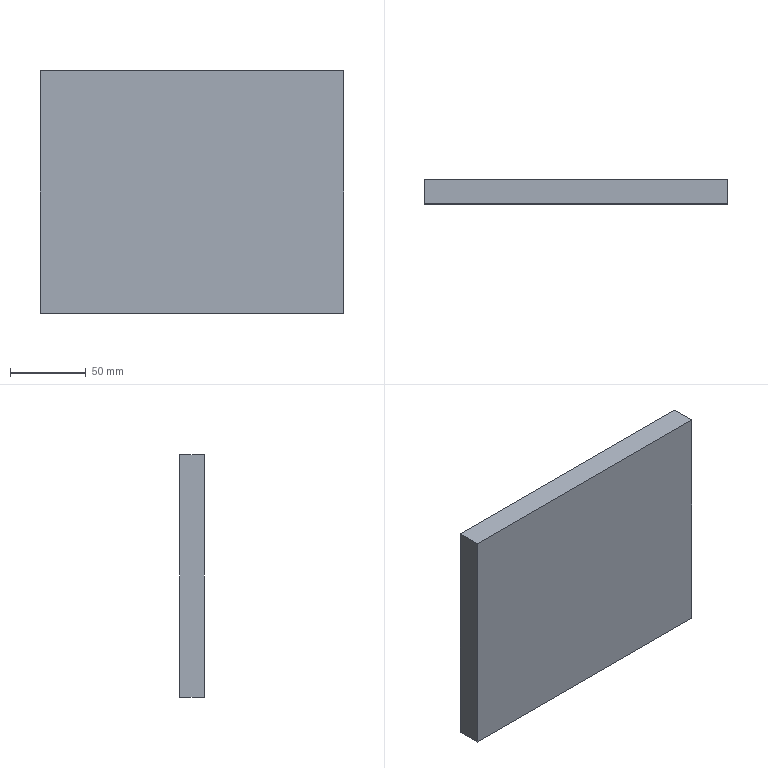Part | STEP file | HJDX-000 | 1 solid | 6 faces | box 200 x 16 x 160 mm | volume 512000 mm3 | plane 6
STEP:
#1=CARTESIAN_POINT('',(-100.,16.,-80.));
#2=VERTEX_POINT('',#1);
#3=CARTESIAN_POINT('',(100.,16.,-80.));
#4=VERTEX_POINT('',#3);
#5=CARTESIAN_POINT('',(0.,16.,-80.));
#6=DIRECTION('',(1.,0.,0.));
#7=VECTOR('',#6,1000.);
#8=LINE('',#5,#7);
#9=EDGE_CURVE('',#2,#4,#8,.T.);
#10=ORIENTED_EDGE('',*,*,#9,.F.);
#11=CARTESIAN_POINT('',(-100.,16.,80.));
#12=VERTEX_POINT('',#11);
#13=CARTESIAN_POINT('',(-100.,16.,0.));
#14=DIRECTION('',(0.,0.,-1.));
#15=VECTOR('',#14,1000.);
#16=LINE('',#13,#15);
#17=EDGE_CURVE('',#12,#2,#16,.T.);
#18=ORIENTED_EDGE('',*,*,#17,.F.);
#19=CARTESIAN_POINT('',(100.,16.,80.));
#20=VERTEX_POINT('',#19);
#21=CARTESIAN_POINT('',(0.,16.,80.));
#22=DIRECTION('',(-1.,0.,0.));
#23=VECTOR('',#22,1000.);
#24=LINE('',#21,#23);
#25=EDGE_CURVE('',#20,#12,#24,.T.);
#26=ORIENTED_EDGE('',*,*,#25,.F.);
#27=CARTESIAN_POINT('',(100.,16.,0.));
#28=DIRECTION('',(0.,0.,1.));
#29=VECTOR('',#28,1000.);
#30=LINE('',#27,#29);
#31=EDGE_CURVE('',#4,#20,#30,.T.);
#32=ORIENTED_EDGE('',*,*,#31,.F.);
#33=EDGE_LOOP('',(#10,#18,#26,#32));
#34=FACE_OUTER_BOUND('',#33,.T.);
#35=CARTESIAN_POINT('',(0.,16.,0.));
#36=DIRECTION('',(0.,-1.,0.));
#37=DIRECTION('',(0.,0.,-1.));
#38=AXIS2_PLACEMENT_3D('',#35,#36,#37);
#39=PLANE('',#38);
#40=ADVANCED_FACE('',(#34),#39,.F.);
#41=CARTESIAN_POINT('',(100.,0.,-80.));
#42=VERTEX_POINT('',#41);
#43=CARTESIAN_POINT('',(100.,16.,-80.));
#44=DIRECTION('',(0.,-1.,0.));
#45=VECTOR('',#44,1000.);
#46=LINE('',#43,#45);
#47=EDGE_CURVE('',#4,#42,#46,.T.);
#48=ORIENTED_EDGE('',*,*,#47,.F.);
#49=ORIENTED_EDGE('',*,*,#31,.T.);
#50=CARTESIAN_POINT('',(100.,0.,80.));
#51=VERTEX_POINT('',#50);
#52=CARTESIAN_POINT('',(100.,16.,80.));
#53=DIRECTION('',(0.,1.,0.));
#54=VECTOR('',#53,1000.);
#55=LINE('',#52,#54);
#56=EDGE_CURVE('',#51,#20,#55,.T.);
#57=ORIENTED_EDGE('',*,*,#56,.F.);
#58=CARTESIAN_POINT('',(100.,0.,80.));
#59=DIRECTION('',(0.,0.,1.));
#60=VECTOR('',#59,1000.);
#61=LINE('',#58,#60);
#62=EDGE_CURVE('',#42,#51,#61,.T.);
#63=ORIENTED_EDGE('',*,*,#62,.F.);
#64=EDGE_LOOP('',(#48,#49,#57,#63));
#65=FACE_OUTER_BOUND('',#64,.T.);
#66=CARTESIAN_POINT('',(100.,16.,80.));
#67=DIRECTION('',(-1.,0.,0.));
#68=DIRECTION('',(0.,0.,1.));
#69=AXIS2_PLACEMENT_3D('',#66,#67,#68);
#70=PLANE('',#69);
#71=ADVANCED_FACE('',(#65),#70,.F.);
#72=CARTESIAN_POINT('',(-100.,0.,-80.));
#73=VERTEX_POINT('',#72);
#74=CARTESIAN_POINT('',(-100.,16.,-80.));
#75=DIRECTION('',(0.,-1.,0.));
#76=VECTOR('',#75,1000.);
#77=LINE('',#74,#76);
#78=EDGE_CURVE('',#2,#73,#77,.T.);
#79=ORIENTED_EDGE('',*,*,#78,.F.);
#80=ORIENTED_EDGE('',*,*,#9,.T.);
#81=ORIENTED_EDGE('',*,*,#47,.T.);
#82=CARTESIAN_POINT('',(-100.,0.,-80.));
#83=DIRECTION('',(1.,0.,0.));
#84=VECTOR('',#83,1000.);
#85=LINE('',#82,#84);
#86=EDGE_CURVE('',#73,#42,#85,.T.);
#87=ORIENTED_EDGE('',*,*,#86,.F.);
#88=EDGE_LOOP('',(#79,#80,#81,#87));
#89=FACE_OUTER_BOUND('',#88,.T.);
#90=CARTESIAN_POINT('',(-100.,16.,-80.));
#91=DIRECTION('',(0.,0.,1.));
#92=DIRECTION('',(1.,0.,0.));
#93=AXIS2_PLACEMENT_3D('',#90,#91,#92);
#94=PLANE('',#93);
#95=ADVANCED_FACE('',(#89),#94,.F.);
#96=CARTESIAN_POINT('',(-100.,0.,80.));
#97=VERTEX_POINT('',#96);
#98=CARTESIAN_POINT('',(-100.,16.,80.));
#99=DIRECTION('',(0.,-1.,0.));
#100=VECTOR('',#99,1000.);
#101=LINE('',#98,#100);
#102=EDGE_CURVE('',#12,#97,#101,.T.);
#103=ORIENTED_EDGE('',*,*,#102,.F.);
#104=ORIENTED_EDGE('',*,*,#17,.T.);
#105=ORIENTED_EDGE('',*,*,#78,.T.);
#106=CARTESIAN_POINT('',(-100.,0.,80.));
#107=DIRECTION('',(0.,0.,-1.));
#108=VECTOR('',#107,1000.);
#109=LINE('',#106,#108);
#110=EDGE_CURVE('',#97,#73,#109,.T.);
#111=ORIENTED_EDGE('',*,*,#110,.F.);
#112=EDGE_LOOP('',(#103,#104,#105,#111));
#113=FACE_OUTER_BOUND('',#112,.T.);
#114=CARTESIAN_POINT('',(-100.,16.,80.));
#115=DIRECTION('',(1.,0.,0.));
#116=DIRECTION('',(0.,0.,-1.));
#117=AXIS2_PLACEMENT_3D('',#114,#115,#116);
#118=PLANE('',#117);
#119=ADVANCED_FACE('',(#113),#118,.F.);
#120=ORIENTED_EDGE('',*,*,#56,.T.);
#121=ORIENTED_EDGE('',*,*,#25,.T.);
#122=ORIENTED_EDGE('',*,*,#102,.T.);
#123=CARTESIAN_POINT('',(-100.,0.,80.));
#124=DIRECTION('',(-1.,0.,0.));
#125=VECTOR('',#124,1000.);
#126=LINE('',#123,#125);
#127=EDGE_CURVE('',#51,#97,#126,.T.);
#128=ORIENTED_EDGE('',*,*,#127,.F.);
#129=EDGE_LOOP('',(#120,#121,#122,#128));
#130=FACE_OUTER_BOUND('',#129,.T.);
#131=CARTESIAN_POINT('',(-100.,16.,80.));
#132=DIRECTION('',(0.,0.,-1.));
#133=DIRECTION('',(-1.,0.,0.));
#134=AXIS2_PLACEMENT_3D('',#131,#132,#133);
#135=PLANE('',#134);
#136=ADVANCED_FACE('',(#130),#135,.F.);
#137=ORIENTED_EDGE('',*,*,#110,.T.);
#138=ORIENTED_EDGE('',*,*,#86,.T.);
#139=ORIENTED_EDGE('',*,*,#62,.T.);
#140=ORIENTED_EDGE('',*,*,#127,.T.);
#141=EDGE_LOOP('',(#137,#138,#139,#140));
#142=FACE_OUTER_BOUND('',#141,.T.);
#143=CARTESIAN_POINT('',(0.,0.,0.));
#144=DIRECTION('',(0.,-1.,0.));
#145=DIRECTION('',(0.,0.,-1.));
#146=AXIS2_PLACEMENT_3D('',#143,#144,#145);
#147=PLANE('',#146);
#148=ADVANCED_FACE('',(#142),#147,.T.);
#149=CLOSED_SHELL('',(#40,#71,#95,#119,#136,#148));
#150=MANIFOLD_SOLID_BREP('',#149);
#151=CARTESIAN_POINT('',(0.,0.,0.));
#152=DIRECTION('',(0.,0.,1.));
#153=DIRECTION('',(1.,0.,0.));
#154=AXIS2_PLACEMENT_3D('',#151,#152,#153);
#155=(LENGTH_UNIT()NAMED_UNIT(*)SI_UNIT(.MILLI.,.METRE.));
#156=UNCERTAINTY_MEASURE_WITH_UNIT(LENGTH_MEASURE(0.00001),#155,'','');
#157=(NAMED_UNIT(*)PLANE_ANGLE_UNIT()SI_UNIT($,.RADIAN.));
#158=(NAMED_UNIT(*)SI_UNIT($,.STERADIAN.)SOLID_ANGLE_UNIT());
#159=(GEOMETRIC_REPRESENTATION_CONTEXT(3)GLOBAL_UNCERTAINTY_ASSIGNED_CONTEXT((#156))GLOBAL_UNIT_ASSIGNED_CONTEXT((#155,#157,#158))REPRESENTATION_CONTEXT('',''));
#160=ADVANCED_BREP_SHAPE_REPRESENTATION('',(#150,#154),#159);